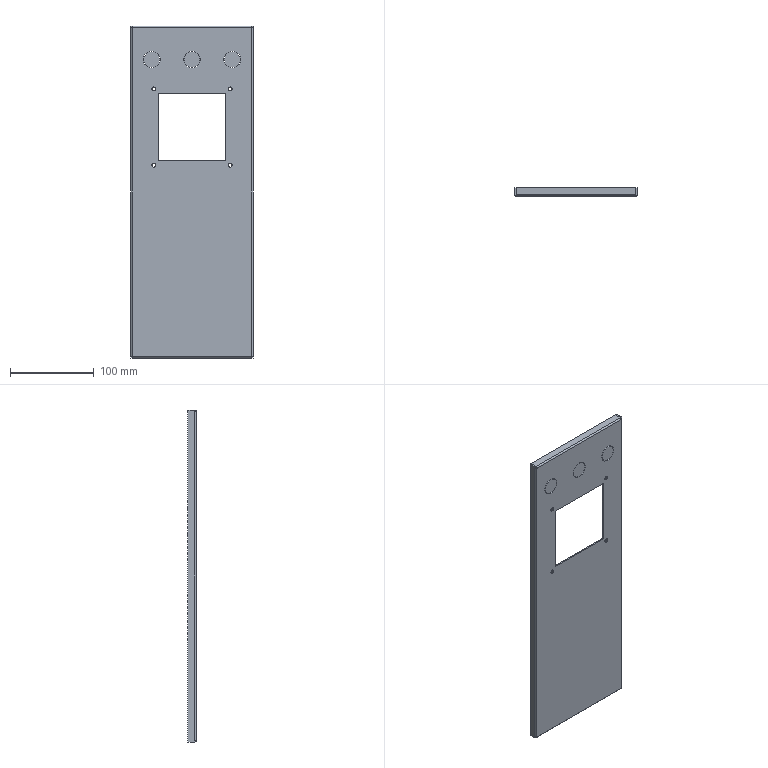Part | SolidWorks | features BaseBody 1 | 1 solid | 74 faces | box 146 x 10 x 396 mm | volume 89690 mm3 | plane 46 | cylinder 28 | commonest cylinder face diameters 4.5 x8 19 x6 20 x6 0.4 x4 3.4 x4